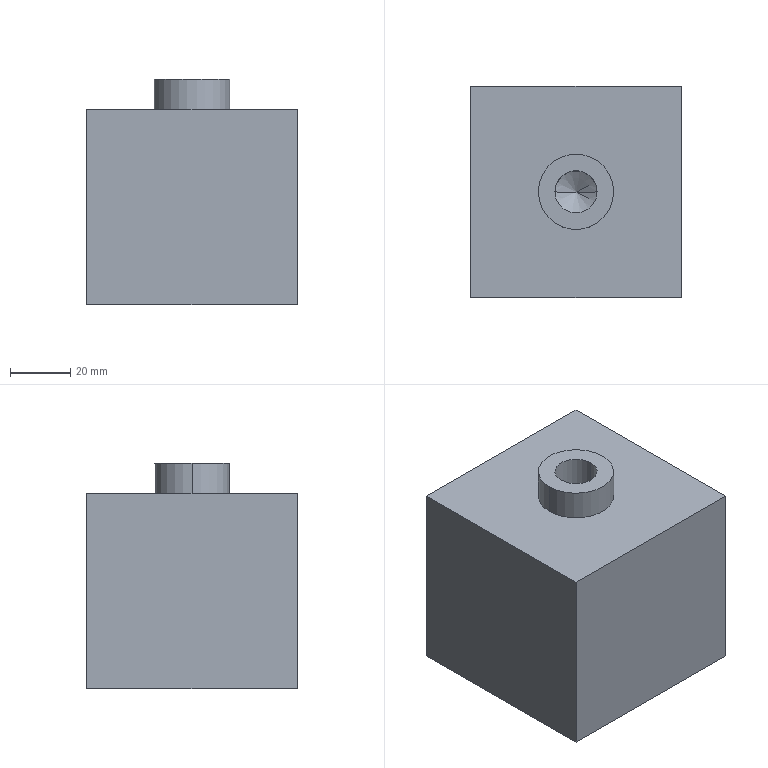Part | SolidWorks | features Extrusion 1, HoleWzd 1, ICE 1 | 1 solid | 13 faces | box 70 x 70 x 75 mm | volume 316728 mm3 | plane 7 | cylinder 4 | cone 2 | commonest cylinder face diameters 14 x2 25 x2
STEP:
#1=CARTESIAN_POINT('',(-7.,0.,33.));
#2=VERTEX_POINT('',#1);
#3=CARTESIAN_POINT('',(7.,0.,33.));
#4=VERTEX_POINT('',#3);
#5=CARTESIAN_POINT('',(0.,0.,33.));
#6=DIRECTION('',(0.,0.,1.));
#7=DIRECTION('',(1.,0.,0.));
#8=AXIS2_PLACEMENT_3D('',#5,#6,#7);
#9=CIRCLE('',#8,7.);
#10=EDGE_CURVE('',#2,#4,#9,.T.);
#11=ORIENTED_EDGE('',*,*,#10,.F.);
#12=CARTESIAN_POINT('',(-7.,0.,75.));
#13=VERTEX_POINT('',#12);
#14=CARTESIAN_POINT('',(-7.,0.,75.));
#15=DIRECTION('',(0.,0.,1.));
#16=VECTOR('',#15,1000.);
#17=LINE('',#14,#16);
#18=EDGE_CURVE('',#2,#13,#17,.T.);
#19=ORIENTED_EDGE('',*,*,#18,.T.);
#20=CARTESIAN_POINT('',(7.,0.,75.));
#21=VERTEX_POINT('',#20);
#22=CARTESIAN_POINT('',(0.,0.,75.));
#23=DIRECTION('',(0.,0.,1.));
#24=DIRECTION('',(1.,0.,0.));
#25=AXIS2_PLACEMENT_3D('',#22,#23,#24);
#26=CIRCLE('',#25,7.);
#27=EDGE_CURVE('',#13,#21,#26,.T.);
#28=ORIENTED_EDGE('',*,*,#27,.T.);
#29=CARTESIAN_POINT('',(7.,0.,75.));
#30=DIRECTION('',(0.,0.,1.));
#31=VECTOR('',#30,1000.);
#32=LINE('',#29,#31);
#33=EDGE_CURVE('',#4,#21,#32,.T.);
#34=ORIENTED_EDGE('',*,*,#33,.F.);
#35=EDGE_LOOP('',(#11,#19,#28,#34));
#36=FACE_OUTER_BOUND('',#35,.T.);
#37=CARTESIAN_POINT('',(0.,0.,75.));
#38=DIRECTION('',(0.,0.,1.));
#39=DIRECTION('',(1.,0.,0.));
#40=AXIS2_PLACEMENT_3D('',#37,#38,#39);
#41=CYLINDRICAL_SURFACE('',#40,7.);
#42=ADVANCED_FACE('',(#36),#41,.F.);
#43=CARTESIAN_POINT('',(0.,0.,28.794));
#44=VERTEX_POINT('',#43);
#45=CARTESIAN_POINT('',(7.,0.,33.));
#46=DIRECTION('',(0.8572,0.,0.515));
#47=VECTOR('',#46,1000.);
#48=LINE('',#45,#47);
#49=EDGE_CURVE('',#44,#4,#48,.T.);
#50=ORIENTED_EDGE('',*,*,#49,.F.);
#51=CARTESIAN_POINT('',(-7.,0.,33.));
#52=DIRECTION('',(-0.8572,0.,0.515));
#53=VECTOR('',#52,1000.);
#54=LINE('',#51,#53);
#55=EDGE_CURVE('',#44,#2,#54,.T.);
#56=ORIENTED_EDGE('',*,*,#55,.T.);
#57=ORIENTED_EDGE('',*,*,#10,.T.);
#58=EDGE_LOOP('',(#50,#56,#57));
#59=FACE_OUTER_BOUND('',#58,.T.);
#60=CARTESIAN_POINT('',(0.,0.,33.));
#61=DIRECTION('',(0.,0.,1.));
#62=DIRECTION('',(1.,0.,0.));
#63=AXIS2_PLACEMENT_3D('',#60,#61,#62);
#64=CONICAL_SURFACE('',#63,7.,1.03);
#65=ADVANCED_FACE('',(#59),#64,.F.);
#66=CARTESIAN_POINT('',(12.5,0.,75.));
#67=VERTEX_POINT('',#66);
#68=CARTESIAN_POINT('',(-12.5,0.,75.));
#69=VERTEX_POINT('',#68);
#70=CARTESIAN_POINT('',(0.,0.,75.));
#71=DIRECTION('',(0.,0.,1.));
#72=DIRECTION('',(1.,0.,0.));
#73=AXIS2_PLACEMENT_3D('',#70,#71,#72);
#74=CIRCLE('',#73,12.5);
#75=EDGE_CURVE('',#67,#69,#74,.T.);
#76=ORIENTED_EDGE('',*,*,#75,.F.);
#77=CARTESIAN_POINT('',(12.5,0.,65.));
#78=VERTEX_POINT('',#77);
#79=CARTESIAN_POINT('',(12.5,0.,75.));
#80=DIRECTION('',(0.,0.,-1.));
#81=VECTOR('',#80,1000.);
#82=LINE('',#79,#81);
#83=EDGE_CURVE('',#67,#78,#82,.T.);
#84=ORIENTED_EDGE('',*,*,#83,.T.);
#85=CARTESIAN_POINT('',(-12.5,0.,65.));
#86=VERTEX_POINT('',#85);
#87=CARTESIAN_POINT('',(0.,0.,65.));
#88=DIRECTION('',(0.,0.,1.));
#89=DIRECTION('',(1.,0.,0.));
#90=AXIS2_PLACEMENT_3D('',#87,#88,#89);
#91=CIRCLE('',#90,12.5);
#92=EDGE_CURVE('',#78,#86,#91,.T.);
#93=ORIENTED_EDGE('',*,*,#92,.T.);
#94=CARTESIAN_POINT('',(-12.5,0.,75.));
#95=DIRECTION('',(0.,0.,-1.));
#96=VECTOR('',#95,1000.);
#97=LINE('',#94,#96);
#98=EDGE_CURVE('',#69,#86,#97,.T.);
#99=ORIENTED_EDGE('',*,*,#98,.F.);
#100=EDGE_LOOP('',(#76,#84,#93,#99));
#101=FACE_OUTER_BOUND('',#100,.T.);
#102=CARTESIAN_POINT('',(0.,0.,75.));
#103=DIRECTION('',(0.,0.,-1.));
#104=DIRECTION('',(-1.,0.,0.));
#105=AXIS2_PLACEMENT_3D('',#102,#103,#104);
#106=CYLINDRICAL_SURFACE('',#105,12.5);
#107=ADVANCED_FACE('',(#101),#106,.T.);
#108=CARTESIAN_POINT('',(-35.,35.,0.));
#109=VERTEX_POINT('',#108);
#110=CARTESIAN_POINT('',(-35.,-35.,0.));
#111=VERTEX_POINT('',#110);
#112=CARTESIAN_POINT('',(-35.,-35.,0.));
#113=DIRECTION('',(0.,-1.,0.));
#114=VECTOR('',#113,1000.);
#115=LINE('',#112,#114);
#116=EDGE_CURVE('',#109,#111,#115,.T.);
#117=ORIENTED_EDGE('',*,*,#116,.T.);
#118=CARTESIAN_POINT('',(-35.,-35.,65.));
#119=VERTEX_POINT('',#118);
#120=CARTESIAN_POINT('',(-35.,-35.,65.));
#121=DIRECTION('',(0.,0.,-1.));
#122=VECTOR('',#121,1000.);
#123=LINE('',#120,#122);
#124=EDGE_CURVE('',#119,#111,#123,.T.);
#125=ORIENTED_EDGE('',*,*,#124,.F.);
#126=CARTESIAN_POINT('',(-35.,35.,65.));
#127=VERTEX_POINT('',#126);
#128=CARTESIAN_POINT('',(-35.,-35.,65.));
#129=DIRECTION('',(0.,-1.,0.));
#130=VECTOR('',#129,1000.);
#131=LINE('',#128,#130);
#132=EDGE_CURVE('',#127,#119,#131,.T.);
#133=ORIENTED_EDGE('',*,*,#132,.F.);
#134=CARTESIAN_POINT('',(-35.,35.,65.));
#135=DIRECTION('',(0.,0.,-1.));
#136=VECTOR('',#135,1000.);
#137=LINE('',#134,#136);
#138=EDGE_CURVE('',#127,#109,#137,.T.);
#139=ORIENTED_EDGE('',*,*,#138,.T.);
#140=EDGE_LOOP('',(#117,#125,#133,#139));
#141=FACE_OUTER_BOUND('',#140,.T.);
#142=CARTESIAN_POINT('',(-35.,-35.,65.));
#143=DIRECTION('',(1.,0.,0.));
#144=DIRECTION('',(0.,0.,-1.));
#145=AXIS2_PLACEMENT_3D('',#142,#143,#144);
#146=PLANE('',#145);
#147=ADVANCED_FACE('',(#141),#146,.F.);
#148=CARTESIAN_POINT('',(35.,-35.,0.));
#149=VERTEX_POINT('',#148);
#150=CARTESIAN_POINT('',(35.,-35.,0.));
#151=DIRECTION('',(1.,0.,0.));
#152=VECTOR('',#151,1000.);
#153=LINE('',#150,#152);
#154=EDGE_CURVE('',#111,#149,#153,.T.);
#155=ORIENTED_EDGE('',*,*,#154,.T.);
#156=CARTESIAN_POINT('',(35.,-35.,65.));
#157=VERTEX_POINT('',#156);
#158=CARTESIAN_POINT('',(35.,-35.,65.));
#159=DIRECTION('',(0.,0.,-1.));
#160=VECTOR('',#159,1000.);
#161=LINE('',#158,#160);
#162=EDGE_CURVE('',#157,#149,#161,.T.);
#163=ORIENTED_EDGE('',*,*,#162,.F.);
#164=CARTESIAN_POINT('',(35.,-35.,65.));
#165=DIRECTION('',(1.,0.,0.));
#166=VECTOR('',#165,1000.);
#167=LINE('',#164,#166);
#168=EDGE_CURVE('',#119,#157,#167,.T.);
#169=ORIENTED_EDGE('',*,*,#168,.F.);
#170=ORIENTED_EDGE('',*,*,#124,.T.);
#171=EDGE_LOOP('',(#155,#163,#169,#170));
#172=FACE_OUTER_BOUND('',#171,.T.);
#173=CARTESIAN_POINT('',(35.,-35.,65.));
#174=DIRECTION('',(0.,1.,0.));
#175=DIRECTION('',(-1.,0.,0.));
#176=AXIS2_PLACEMENT_3D('',#173,#174,#175);
#177=PLANE('',#176);
#178=ADVANCED_FACE('',(#172),#177,.F.);
#179=CARTESIAN_POINT('',(35.,35.,0.));
#180=VERTEX_POINT('',#179);
#181=CARTESIAN_POINT('',(35.,-35.,0.));
#182=DIRECTION('',(0.,1.,0.));
#183=VECTOR('',#182,1000.);
#184=LINE('',#181,#183);
#185=EDGE_CURVE('',#149,#180,#184,.T.);
#186=ORIENTED_EDGE('',*,*,#185,.T.);
#187=CARTESIAN_POINT('',(35.,35.,65.));
#188=VERTEX_POINT('',#187);
#189=CARTESIAN_POINT('',(35.,35.,65.));
#190=DIRECTION('',(0.,0.,-1.));
#191=VECTOR('',#190,1000.);
#192=LINE('',#189,#191);
#193=EDGE_CURVE('',#188,#180,#192,.T.);
#194=ORIENTED_EDGE('',*,*,#193,.F.);
#195=CARTESIAN_POINT('',(35.,-35.,65.));
#196=DIRECTION('',(0.,1.,0.));
#197=VECTOR('',#196,1000.);
#198=LINE('',#195,#197);
#199=EDGE_CURVE('',#157,#188,#198,.T.);
#200=ORIENTED_EDGE('',*,*,#199,.F.);
#201=ORIENTED_EDGE('',*,*,#162,.T.);
#202=EDGE_LOOP('',(#186,#194,#200,#201));
#203=FACE_OUTER_BOUND('',#202,.T.);
#204=CARTESIAN_POINT('',(35.,-35.,65.));
#205=DIRECTION('',(-1.,0.,0.));
#206=DIRECTION('',(0.,0.,1.));
#207=AXIS2_PLACEMENT_3D('',#204,#205,#206);
#208=PLANE('',#207);
#209=ADVANCED_FACE('',(#203),#208,.F.);
#210=CARTESIAN_POINT('',(35.,35.,0.));
#211=DIRECTION('',(-1.,0.,0.));
#212=VECTOR('',#211,1000.);
#213=LINE('',#210,#212);
#214=EDGE_CURVE('',#180,#109,#213,.T.);
#215=ORIENTED_EDGE('',*,*,#214,.T.);
#216=ORIENTED_EDGE('',*,*,#138,.F.);
#217=CARTESIAN_POINT('',(35.,35.,65.));
#218=DIRECTION('',(-1.,0.,0.));
#219=VECTOR('',#218,1000.);
#220=LINE('',#217,#219);
#221=EDGE_CURVE('',#188,#127,#220,.T.);
#222=ORIENTED_EDGE('',*,*,#221,.F.);
#223=ORIENTED_EDGE('',*,*,#193,.T.);
#224=EDGE_LOOP('',(#215,#216,#222,#223));
#225=FACE_OUTER_BOUND('',#224,.T.);
#226=CARTESIAN_POINT('',(35.,35.,65.));
#227=DIRECTION('',(0.,-1.,0.));
#228=DIRECTION('',(1.,0.,0.));
#229=AXIS2_PLACEMENT_3D('',#226,#227,#228);
#230=PLANE('',#229);
#231=ADVANCED_FACE('',(#225),#230,.F.);
#232=CARTESIAN_POINT('',(0.,0.,65.));
#233=DIRECTION('',(0.,0.,1.));
#234=DIRECTION('',(1.,0.,0.));
#235=AXIS2_PLACEMENT_3D('',#232,#233,#234);
#236=CIRCLE('',#235,12.5);
#237=EDGE_CURVE('',#86,#78,#236,.T.);
#238=ORIENTED_EDGE('',*,*,#237,.F.);
#239=ORIENTED_EDGE('',*,*,#92,.F.);
#240=EDGE_LOOP('',(#238,#239));
#241=FACE_BOUND('',#240,.T.);
#242=ORIENTED_EDGE('',*,*,#132,.T.);
#243=ORIENTED_EDGE('',*,*,#168,.T.);
#244=ORIENTED_EDGE('',*,*,#199,.T.);
#245=ORIENTED_EDGE('',*,*,#221,.T.);
#246=EDGE_LOOP('',(#242,#243,#244,#245));
#247=FACE_OUTER_BOUND('',#246,.T.);
#248=CARTESIAN_POINT('',(0.,0.,65.));
#249=DIRECTION('',(0.,0.,1.));
#250=DIRECTION('',(1.,0.,0.));
#251=AXIS2_PLACEMENT_3D('',#248,#249,#250);
#252=PLANE('',#251);
#253=ADVANCED_FACE('',(#241,#247),#252,.T.);
#254=ORIENTED_EDGE('',*,*,#116,.F.);
#255=ORIENTED_EDGE('',*,*,#214,.F.);
#256=ORIENTED_EDGE('',*,*,#185,.F.);
#257=ORIENTED_EDGE('',*,*,#154,.F.);
#258=EDGE_LOOP('',(#254,#255,#256,#257));
#259=FACE_OUTER_BOUND('',#258,.T.);
#260=CARTESIAN_POINT('',(0.,0.,0.));
#261=DIRECTION('',(0.,0.,1.));
#262=DIRECTION('',(1.,0.,0.));
#263=AXIS2_PLACEMENT_3D('',#260,#261,#262);
#264=PLANE('',#263);
#265=ADVANCED_FACE('',(#259),#264,.F.);
#266=ORIENTED_EDGE('',*,*,#83,.F.);
#267=CARTESIAN_POINT('',(0.,0.,75.));
#268=DIRECTION('',(0.,0.,1.));
#269=DIRECTION('',(1.,0.,0.));
#270=AXIS2_PLACEMENT_3D('',#267,#268,#269);
#271=CIRCLE('',#270,12.5);
#272=EDGE_CURVE('',#69,#67,#271,.T.);
#273=ORIENTED_EDGE('',*,*,#272,.F.);
#274=ORIENTED_EDGE('',*,*,#98,.T.);
#275=ORIENTED_EDGE('',*,*,#237,.T.);
#276=EDGE_LOOP('',(#266,#273,#274,#275));
#277=FACE_OUTER_BOUND('',#276,.T.);
#278=CARTESIAN_POINT('',(0.,0.,75.));
#279=DIRECTION('',(0.,0.,-1.));
#280=DIRECTION('',(-1.,0.,0.));
#281=AXIS2_PLACEMENT_3D('',#278,#279,#280);
#282=CYLINDRICAL_SURFACE('',#281,12.5);
#283=ADVANCED_FACE('',(#277),#282,.T.);
#284=CARTESIAN_POINT('',(0.,0.,75.));
#285=DIRECTION('',(0.,0.,1.));
#286=DIRECTION('',(1.,0.,0.));
#287=AXIS2_PLACEMENT_3D('',#284,#285,#286);
#288=CIRCLE('',#287,7.);
#289=EDGE_CURVE('',#21,#13,#288,.T.);
#290=ORIENTED_EDGE('',*,*,#289,.F.);
#291=ORIENTED_EDGE('',*,*,#27,.F.);
#292=EDGE_LOOP('',(#290,#291));
#293=FACE_BOUND('',#292,.T.);
#294=ORIENTED_EDGE('',*,*,#272,.T.);
#295=ORIENTED_EDGE('',*,*,#75,.T.);
#296=EDGE_LOOP('',(#294,#295));
#297=FACE_OUTER_BOUND('',#296,.T.);
#298=CARTESIAN_POINT('',(0.,0.,75.));
#299=DIRECTION('',(0.,0.,1.));
#300=DIRECTION('',(1.,0.,0.));
#301=AXIS2_PLACEMENT_3D('',#298,#299,#300);
#302=PLANE('',#301);
#303=ADVANCED_FACE('',(#293,#297),#302,.T.);
#304=ORIENTED_EDGE('',*,*,#55,.F.);
#305=ORIENTED_EDGE('',*,*,#49,.T.);
#306=CARTESIAN_POINT('',(0.,0.,33.));
#307=DIRECTION('',(0.,0.,1.));
#308=DIRECTION('',(1.,0.,0.));
#309=AXIS2_PLACEMENT_3D('',#306,#307,#308);
#310=CIRCLE('',#309,7.);
#311=EDGE_CURVE('',#4,#2,#310,.T.);
#312=ORIENTED_EDGE('',*,*,#311,.T.);
#313=EDGE_LOOP('',(#304,#305,#312));
#314=FACE_OUTER_BOUND('',#313,.T.);
#315=CARTESIAN_POINT('',(0.,0.,33.));
#316=DIRECTION('',(0.,0.,1.));
#317=DIRECTION('',(1.,0.,0.));
#318=AXIS2_PLACEMENT_3D('',#315,#316,#317);
#319=CONICAL_SURFACE('',#318,7.,1.03);
#320=ADVANCED_FACE('',(#314),#319,.F.);
#321=ORIENTED_EDGE('',*,*,#18,.F.);
#322=ORIENTED_EDGE('',*,*,#311,.F.);
#323=ORIENTED_EDGE('',*,*,#33,.T.);
#324=ORIENTED_EDGE('',*,*,#289,.T.);
#325=EDGE_LOOP('',(#321,#322,#323,#324));
#326=FACE_OUTER_BOUND('',#325,.T.);
#327=CARTESIAN_POINT('',(0.,0.,75.));
#328=DIRECTION('',(0.,0.,1.));
#329=DIRECTION('',(1.,0.,0.));
#330=AXIS2_PLACEMENT_3D('',#327,#328,#329);
#331=CYLINDRICAL_SURFACE('',#330,7.);
#332=ADVANCED_FACE('',(#326),#331,.F.);
#333=CLOSED_SHELL('',(#42,#65,#107,#147,#178,#209,#231,#253,#265,#283,#303,#320,#332));
#334=MANIFOLD_SOLID_BREP('',#333);
#335=CARTESIAN_POINT('',(0.,0.,0.));
#336=DIRECTION('',(0.,0.,1.));
#337=DIRECTION('',(1.,0.,0.));
#338=AXIS2_PLACEMENT_3D('',#335,#336,#337);
#339=(LENGTH_UNIT()NAMED_UNIT(*)SI_UNIT(.MILLI.,.METRE.));
#340=UNCERTAINTY_MEASURE_WITH_UNIT(LENGTH_MEASURE(0.00001),#339,'','');
#341=(NAMED_UNIT(*)PLANE_ANGLE_UNIT()SI_UNIT($,.RADIAN.));
#342=(NAMED_UNIT(*)SI_UNIT($,.STERADIAN.)SOLID_ANGLE_UNIT());
#343=(GEOMETRIC_REPRESENTATION_CONTEXT(3)GLOBAL_UNCERTAINTY_ASSIGNED_CONTEXT((#340))GLOBAL_UNIT_ASSIGNED_CONTEXT((#339,#341,#342))REPRESENTATION_CONTEXT('',''));
#344=ADVANCED_BREP_SHAPE_REPRESENTATION('',(#334,#338),#343);